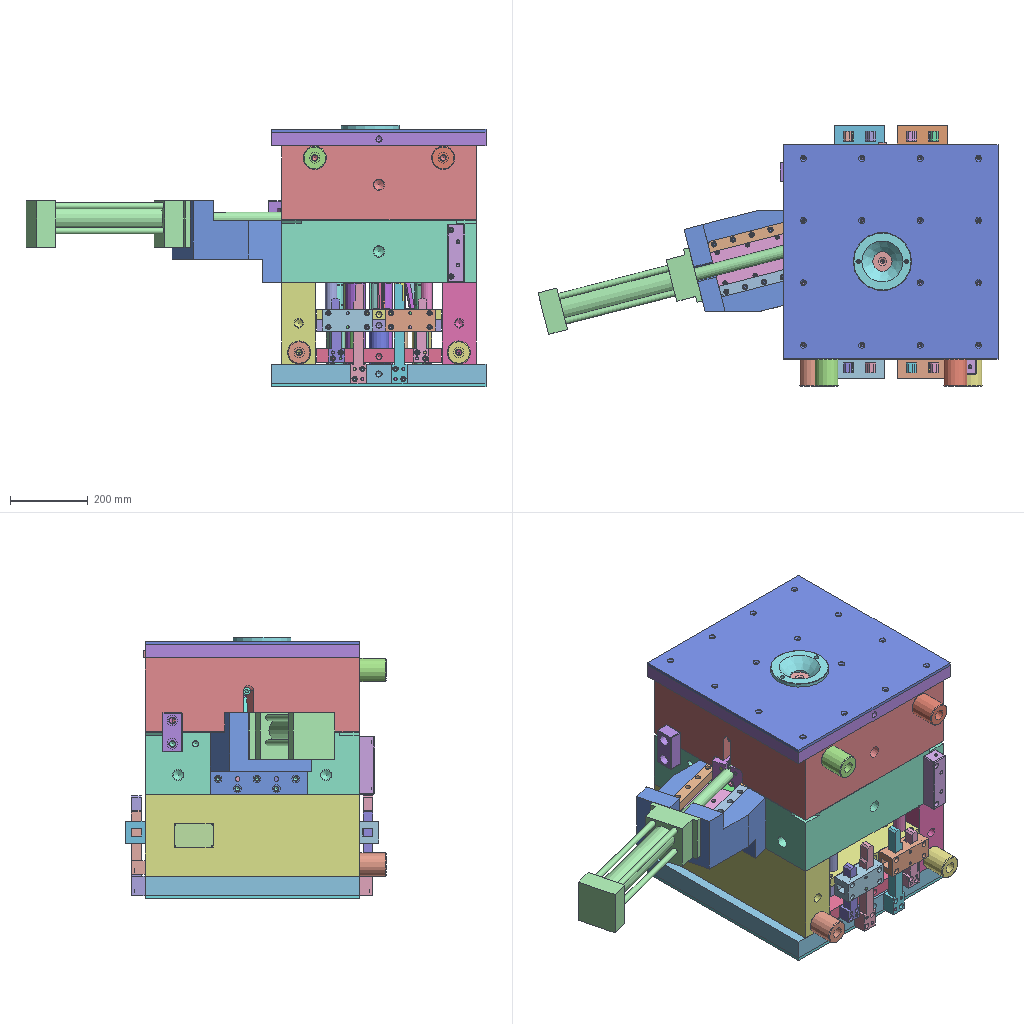Assembly | STEP file | 180 different items | 180 placed | box 1182 x 670 x 672 mm
Parts list (item | name | quantity | size | volume):
1 | stop_rings_id14_x_t | x1 | 20 x 20 x 5 mm | 1313 mm3
2 | stop_rings_id370_x_t | x1 | 20 x 20 x 5 mm | 1313 mm3
3 | stop_rings_id594_x_t | x1 | 20 x 20 x 5 mm | 1313 mm3
4 | stop_rings_id98_x_t | x1 | 20 x 20 x 5 mm | 1313 mm3
5 | 车灯-后视镜_id102_x_t | x1 | 9.556 x 9.556 x 88.278 mm | 4490 mm3
6 | 车灯-后视镜_id106_x_t | x1 | 320 x 550 x 25 mm | 3596280 mm3
7 | 车灯-后视镜_id10_x_t | x1 | 72 x 31.93 x 179.239 mm | 38387 mm3
8 | 车灯-后视镜_id110_x_t | x1 | 129 x 50 x 56 mm | 226318 mm3
9 | 车灯-后视镜_id114_x_t | x1 | 134.693 x 54.944 x 30.493 mm | 17624 mm3
10 | 车灯-后视镜_id118_x_t | x1 | 8 x 50 x 8 mm | 2507 mm3
11 | 车灯-后视镜_id122_x_t | x1 | 100 x 30 x 22 mm | 49982 mm3
12 | 车灯-后视镜_id126_x_t | x1 | 131.992 x 61.149 x 25 mm | 85679 mm3
13 | 车灯-后视镜_id130_x_t | x1 | 61 x 61 x 190 mm | 217774 mm3
14 | 车灯-后视镜_id134_x_t | x1 | 8 x 50 x 8 mm | 2507 mm3
15 | 车灯-后视镜_id138_x_t | x1 | 54.498 x 54.966 x 10 mm | 23790 mm3
16 | 车灯-后视镜_id142_x_t | x1 | 119.383 x 46.093 x 19.5 mm | 38380 mm3
17 | 车灯-后视镜_id146_x_t | x1 | 35 x 35 x 266 mm | 189704 mm3
18 | 车灯-后视镜_id150_x_t | x1 | 8 x 65 x 8 mm | 3261 mm3
19 | 车灯-后视镜_id154_x_t | x1 | 50 x 50 x 85 mm | 164490 mm3
20 | 车灯-后视镜_id158_x_t | x1 | 50.025 x 57.447 x 20 mm | 38834 mm3
21 | 车灯-后视镜_id162_x_t | x1 | 40 x 35 x 257 mm | 187577 mm3
22 | 车灯-后视镜_id166_x_t | x1 | 48 x 48 x 33 mm | 27966 mm3
23 | 车灯-后视镜_id170_x_t | x1 | 9.556 x 9.556 x 94.778 mm | 4817 mm3
24 | 车灯-后视镜_id174_x_t | x1 | 45 x 45 x 330 mm | 416787 mm3
25 | 车灯-后视镜_id178_x_t | x1 | 129 x 50 x 56 mm | 226318 mm3
26 | 车灯-后视镜_id182_x_t | x1 | 48.889 x 38.111 x 25.8 mm | 22170 mm3
27 | 车灯-后视镜_id186_x_t | x1 | 8 x 50 x 8 mm | 2507 mm3
28 | 车灯-后视镜_id18_x_t | x1 | 40 x 40 x 210 mm | 261823 mm3
29 | 车灯-后视镜_id190_x_t | x1 | 100 x 30 x 16.5 mm | 35524 mm3
30 | 车灯-后视镜_id194_x_t | x1 | 192.29 x 72.898 x 25 mm | 123539 mm3
31 | 车灯-后视镜_id198_x_t | x1 | 122.477 x 248.122 x 87.358 mm | 134816 mm3
32 | 车灯-后视镜_id202_x_t | x1 | 8 x 50 x 8 mm | 2507 mm3
33 | 车灯-后视镜_id206_x_t | x1 | 31.448 x 10.108 x 8 mm | 1557 mm3
34 | 车灯-后视镜_id210_x_t | x1 | 119.383 x 46.093 x 27 mm | 44427 mm3
35 | 车灯-后视镜_id214_x_t | x1 | 40 x 40 x 285 mm | 273765 mm3
36 | 车灯-后视镜_id218_x_t | x1 | 8 x 65 x 8 mm | 3261 mm3
37 | 车灯-后视镜_id222_x_t | x1 | 50 x 50 x 85 mm | 164490 mm3
38 | 车灯-后视镜_id226_x_t | x1 | 54.406 x 53.469 x 20 mm | 39812 mm3
39 | 车灯-后视镜_id22_x_t | x1 | 50 x 50 x 85 mm | 164490 mm3
40 | 车灯-后视镜_id230_x_t | x1 | 40 x 35 x 165 mm | 113527 mm3
41 | 车灯-后视镜_id234_x_t | x1 | 35 x 35 x 266 mm | 189704 mm3
42 | 车灯-后视镜_id238_x_t | x1 | 340.675 x 161.916 x 145 mm | 1865094 mm3
43 | 车灯-后视镜_id242_x_t | x1 | 54 x 54 x 53 mm | 49426 mm3
44 | 车灯-后视镜_id246_x_t | x1 | 129 x 50 x 56 mm | 226318 mm3
45 | 车灯-后视镜_id250_x_t | x1 | 180.044 x 59.602 x 42.214 mm | 28311 mm3
46 | 车灯-后视镜_id254_x_t | x1 | 8 x 65 x 8 mm | 3261 mm3
47 | 车灯-后视镜_id258_x_t | x1 | 25 x 50 x 18 mm | 16008 mm3
48 | 车灯-后视镜_id262_x_t | x1 | 226.748 x 84.296 x 25 mm | 147489 mm3
49 | 车灯-后视镜_id266_x_t | x1 | 8 x 50 x 8 mm | 2507 mm3
50 | 车灯-后视镜_id26_x_t | x1 | 84.183 x 23.326 x 319.699 mm | 124323 mm3
51 | 车灯-后视镜_id270_x_t | x1 | 36.435 x 10.457 x 8 mm | 1807 mm3
52 | 车灯-后视镜_id274_x_t | x1 | 33.319 x 37.519 x 48.057 mm | 14519 mm3
53 | 车灯-后视镜_id278_x_t | x1 | 48 x 48 x 33 mm | 27966 mm3
54 | 车灯-后视镜_id282_x_t | x1 | 8 x 65 x 8 mm | 3261 mm3
55 | 车灯-后视镜_id286_x_t | x1 | 50 x 50 x 210 mm | 409927 mm3
56 | 车灯-后视镜_id290_x_t | x1 | 64.479 x 55.577 x 20 mm | 48278 mm3
57 | 车灯-后视镜_id294_x_t | x1 | 122.477 x 248.122 x 87.358 mm | 134767 mm3
58 | 车灯-后视镜_id298_x_t | x1 | 149.9 x 149.9 x 33 mm | 429222 mm3
59 | 车灯-后视镜_id302_x_t | x1 | 40 x 35 x 165 mm | 113527 mm3
60 | 车灯-后视镜_id306_x_t | x1 | 40 x 40 x 285 mm | 273765 mm3
61 | 车灯-后视镜_id30_x_t | x1 | 54 x 54 x 53 mm | 49426 mm3
62 | 车灯-后视镜_id310_x_t | x1 | 80 x 12 x 12 mm | 9048 mm3
63 | 车灯-后视镜_id314_x_t | x1 | 45 x 45 x 330 mm | 416787 mm3
64 | 车灯-后视镜_id318_x_t | x1 | 40 x 35 x 165 mm | 113527 mm3
65 | 车灯-后视镜_id322_x_t | x1 | 81.604 x 38.677 x 31.456 mm | 5262 mm3
66 | 车灯-后视镜_id326_x_t | x1 | 8 x 50 x 8 mm | 2507 mm3
67 | 车灯-后视镜_id330_x_t | x1 | 30 x 100 x 16.5 mm | 35524 mm3
68 | 车灯-后视镜_id334_x_t | x1 | 178.639 x 104.251 x 61.239 mm | 236319 mm3
69 | 车灯-后视镜_id338_x_t | x1 | 8 x 50 x 8 mm | 2507 mm3
70 | 车灯-后视镜_id342_x_t | x1 | 10.152 x 35.922 x 8 mm | 1784 mm3
71 | 车灯-后视镜_id346_x_t | x1 | 8 x 8 x 16 mm | 739.323 mm3
72 | 车灯-后视镜_id34_x_t | x1 | 182.446 x 54.425 x 9.706 mm | 9470 mm3
73 | 车灯-后视镜_id350_x_t | x1 | 48 x 48 x 33 mm | 27966 mm3
74 | 车灯-后视镜_id354_x_t | x1 | 8 x 50 x 8 mm | 2507 mm3
75 | 车灯-后视镜_id358_x_t | x1 | 50 x 50 x 210 mm | 409927 mm3
76 | 车灯-后视镜_id362_x_t | x1 | 50.625 x 37.635 x 28 mm | 23645 mm3
77 | 车灯-后视镜_id366_x_t | x1 | - | 9620612 mm3
78 | 车灯-后视镜_id374_x_t | x1 | 44 x 40 x 150 mm | 242093 mm3
79 | 车灯-后视镜_id378_x_t | x1 | 35 x 25 x 20 mm | 16780 mm3
80 | 车灯-后视镜_id382_x_t | x1 | 40 x 40 x 285 mm | 273765 mm3
81 | 车灯-后视镜_id386_x_t | x1 | 80 x 12 x 12 mm | 9048 mm3
82 | 车灯-后视镜_id38_x_t | x1 | 320 x 550 x 30 mm | 4485754 mm3
83 | 车灯-后视镜_id390_x_t | x1 | 54 x 54 x 53 mm | 49426 mm3
84 | 车灯-后视镜_id394_x_t | x1 | 40 x 35 x 165 mm | 113527 mm3
85 | 车灯-后视镜_id398_x_t | x1 | 259.149 x 112.453 x 94.778 mm | 42702 mm3
86 | 车灯-后视镜_id402_x_t | x1 | 6.332 x 10 x 315.5 mm | 6416 mm3
87 | 车灯-后视镜_id406_x_t | x1 | 30 x 100 x 16.5 mm | 35524 mm3
88 | 车灯-后视镜_id410_x_t | x1 | 133.87 x 99.984 x 67.76 mm | 199506 mm3
89 | 车灯-后视镜_id414_x_t | x1 | 8 x 65 x 8 mm | 3261 mm3
90 | 车灯-后视镜_id418_x_t | x1 | 8.91 x 32.338 x 7 mm | 1230 mm3
91 | 车灯-后视镜_id422_x_t | x1 | 688.746 x 238.169 x 120 mm | 2911913 mm3
92 | 车灯-后视镜_id426_x_t | x1 | 45 x 45 x 330 mm | 416787 mm3
93 | 车灯-后视镜_id42_x_t | x1 | 129 x 50 x 56 mm | 226318 mm3
94 | 车灯-后视镜_id430_x_t | x1 | 8 x 50 x 8 mm | 2507 mm3
95 | 车灯-后视镜_id434_x_t | x1 | 50 x 50 x 210 mm | 409927 mm3
96 | 车灯-后视镜_id438_x_t | x1 | 44.639 x 37.217 x 28 mm | 22385 mm3
97 | 车灯-后视镜_id442_x_t | x1 | 197.778 x 377 x 123 mm | 135916 mm3
98 | 车灯-后视镜_id446_x_t | x1 | 35 x 35 x 266 mm | 189704 mm3
99 | 车灯-后视镜_id450_x_t | x1 | 60 x 70 x 60 mm | 173692 mm3
100 | 车灯-后视镜_id454_x_t | x1 | 35 x 25 x 20 mm | 16780 mm3
101 | 车灯-后视镜_id458_x_t | x1 | 45 x 45 x 330 mm | 416787 mm3
102 | 车灯-后视镜_id462_x_t | x1 | 53.642 x 50.81 x 378.343 mm | 173095 mm3
103 | 车灯-后视镜_id466_x_t | x1 | 550 x 550 x 50 mm | 14539056 mm3
104 | 车灯-后视镜_id46_x_t | x1 | 32.198 x 38.885 x 23 mm | 17479 mm3
105 | 车灯-后视镜_id470_x_t | x1 | 40 x 35 x 257 mm | 187577 mm3
106 | 车灯-后视镜_id474_x_t | x1 | 179.972 x 53.773 x 9.672 mm | 9329 mm3
107 | 车灯-后视镜_id478_x_t | x1 | 281.237 x 377 x 129.698 mm | 171076 mm3
108 | 车灯-后视镜_id482_x_t | x1 | 35 x 35 x 80 mm | 41432 mm3
109 | 车灯-后视镜_id486_x_t | x1 | 167.24 x 56.347 x 33.937 mm | 25779 mm3
110 | 车灯-后视镜_id490_x_t | x1 | 8 x 50 x 8 mm | 2507 mm3
111 | 车灯-后视镜_id494_x_t | x1 | 100 x 30 x 22 mm | 49982 mm3
112 | 车灯-后视镜_id498_x_t | x1 | 281.721 x 260 x 210 mm | 5973033 mm3
113 | 车灯-后视镜_id502_x_t | x1 | 500 x 550 x 190 mm | 33080670 mm3
114 | 车灯-后视镜_id506_x_t | x1 | 8 x 50 x 8 mm | 2507 mm3
115 | 车灯-后视镜_id50_x_t | x1 | 8 x 50 x 8 mm | 2507 mm3
116 | 车灯-后视镜_id510_x_t | x1 | 50 x 50 x 210 mm | 409927 mm3
117 | 车灯-后视镜_id514_x_t | x1 | 37.194 x 48.439 x 28 mm | 23466 mm3
118 | 车灯-后视镜_id518_x_t | x1 | 280 x 161 x 111 mm | 104739 mm3
119 | 车灯-后视镜_id522_x_t | x1 | 88 x 550 x 210 mm | 9957650 mm3
120 | 车灯-后视镜_id526_x_t | x1 | 60 x 70 x 60 mm | 173692 mm3
121 | 车灯-后视镜_id530_x_t | x1 | 35 x 25 x 20 mm | 16780 mm3
122 | 车灯-后视镜_id534_x_t | x1 | 21.278 x 54.656 x 325.478 mm | 91960 mm3
123 | 车灯-后视镜_id538_x_t | x1 | 40 x 40 x 285 mm | 273765 mm3
124 | 车灯-后视镜_id542_x_t | x1 | 40 x 35 x 257 mm | 187577 mm3
125 | 车灯-后视镜_id546_x_t | x1 | 125.408 x 39.857 x 9.556 mm | 6500 mm3
126 | 车灯-后视镜_id54_x_t | x1 | 100 x 30 x 16.5 mm | 35524 mm3
127 | 车灯-后视镜_id550_x_t | x1 | 280 x 377 x 150.384 mm | 11421529 mm3
128 | 车灯-后视镜_id554_x_t | x1 | 35 x 35 x 80 mm | 41432 mm3
129 | 车灯-后视镜_id558_x_t | x1 | 73.047 x 36.358 x 27.14 mm | 5259 mm3
130 | 车灯-后视镜_id562_x_t | x1 | 8 x 50 x 8 mm | 2507 mm3
131 | 车灯-后视镜_id566_x_t | x1 | 30 x 100 x 22 mm | 49982 mm3
132 | 车灯-后视镜_id570_x_t | x1 | 56.564 x 86.901 x 79.724 mm | 59028 mm3
133 | 车灯-后视镜_id574_x_t | x1 | 61 x 61 x 190 mm | 217774 mm3
134 | 车灯-后视镜_id578_x_t | x1 | 8 x 50 x 8 mm | 2507 mm3
135 | 车灯-后视镜_id582_x_t | x1 | 550 x 550 x 8 mm | 2264649 mm3
136 | 车灯-后视镜_id586_x_t | x1 | 37.285 x 49.936 x 28 mm | 23540 mm3
137 | 车灯-后视镜_id58_x_t | x1 | 125 x 59.346 x 25 mm | 80625 mm3
138 | 车灯-后视镜_id590_x_t | x1 | 6.638 x 10 x 131.059 mm | 3645 mm3
139 | 车灯-后视镜_id598_x_t | x1 | 60 x 70 x 60 mm | 173692 mm3
140 | 车灯-后视镜_id602_x_t | x1 | 35 x 25 x 20 mm | 16780 mm3
141 | 车灯-后视镜_id606_x_t | x1 | 15.208 x 52.995 x 313.531 mm | 58140 mm3
142 | 车灯-后视镜_id610_x_t | x1 | 48 x 48 x 33 mm | 27966 mm3
143 | 车灯-后视镜_id614_x_t | x1 | 40 x 35 x 257 mm | 187577 mm3
144 | 车灯-后视镜_id618_x_t | x1 | 125.408 x 39.857 x 9.556 mm | 6500 mm3
145 | 车灯-后视镜_id622_x_t | x1 | 500 x 550 x 160 mm | 32899557 mm3
146 | 车灯-后视镜_id626_x_t | x1 | 35 x 35 x 80 mm | 41432 mm3
147 | 车灯-后视镜_id62_x_t | x1 | 61 x 61 x 190 mm | 217774 mm3
148 | 车灯-后视镜_id630_x_t | x1 | 156.791 x 56.039 x 26.254 mm | 19026 mm3
149 | 车灯-后视镜_id634_x_t | x1 | 8 x 65 x 8 mm | 3261 mm3
150 | 车灯-后视镜_id638_x_t | x1 | 30 x 100 x 22 mm | 49982 mm3
151 | 车灯-后视镜_id642_x_t | x1 | 152.531 x 146.332 x 12 mm | 183119 mm3
152 | 车灯-后视镜_id646_x_t | x1 | 550 x 550 x 35 mm | 10040225 mm3
153 | 车灯-后视镜_id650_x_t | x1 | 8 x 50 x 8 mm | 2507 mm3
154 | 车灯-后视镜_id654_x_t | x1 | 550 x 550 x 8 mm | 2381998 mm3
155 | 车灯-后视镜_id658_x_t | x1 | 55.522 x 50.883 x 10 mm | 21930 mm3
156 | 车灯-后视镜_id662_x_t | x1 | 10 x 10 x 138.616 mm | 4062 mm3
157 | 车灯-后视镜_id666_x_t | x1 | 54 x 54 x 53 mm | 49426 mm3
158 | 车灯-后视镜_id66_x_t | x1 | 8 x 65 x 8 mm | 3261 mm3
159 | 车灯-后视镜_id670_x_t | x1 | 60 x 70 x 60 mm | 173692 mm3
160 | 车灯-后视镜_id674_x_t | x1 | 50 x 50 x 85 mm | 164490 mm3
161 | 车灯-后视镜_id678_x_t | x1 | 70.106 x 20.475 x 302.011 mm | 62813 mm3
162 | 车灯-后视镜_id682_x_t | x1 | 88 x 550 x 210 mm | 9957597 mm3
163 | 车灯-后视镜_id686_x_t | x1 | 24.107 x 64.242 x 19.839 mm | 3383 mm3
164 | 车灯-后视镜_id690_x_t | x1 | 320 x 550 x 35 mm | 4960596 mm3
165 | 车灯-后视镜_id694_x_t | x1 | 35 x 35 x 80 mm | 41432 mm3
166 | 车灯-后视镜_id698_x_t | x1 | 64.214 x 40.022 x 86 mm | 109388 mm3
167 | 车灯-后视镜_id6_x_t | x1 | 49.536 x 50.464 x 10 mm | 19050 mm3
168 | 车灯-后视镜_id702_x_t | x1 | 8 x 65 x 8 mm | 3261 mm3
169 | 车灯-后视镜_id706_x_t | x1 | 25 x 50 x 13 mm | 11607 mm3
170 | 车灯-后视镜_id70_x_t | x1 | 35 x 50 x 100 mm | 146008 mm3
171 | 车灯-后视镜_id710_x_t | x1 | 214.417 x 153.693 x 12 mm | 250941 mm3
172 | 车灯-后视镜_id714_x_t | x1 | 61 x 61 x 190 mm | 217774 mm3
173 | 车灯-后视镜_id718_x_t | x1 | 8 x 50 x 8 mm | 2507 mm3
174 | 车灯-后视镜_id722_x_t | x1 | 65 x 337.5 x 148.701 mm | 402158 mm3
175 | 车灯-后视镜_id74_x_t | x1 | 54.406 x 53.469 x 10 mm | 23010 mm3
176 | 车灯-后视镜_id78_x_t | x1 | 143.857 x 68.896 x 72 mm | 222992 mm3
177 | 车灯-后视镜_id82_x_t | x1 | 35 x 35 x 266 mm | 189704 mm3
178 | 车灯-后视镜_id86_x_t | x1 | 0.5 x 100 x 60 mm | 2994 mm3
179 | 车灯-后视镜_id90_x_t | x1 | 50 x 50 x 85 mm | 164490 mm3
180 | 车灯-后视镜_id94_x_t | x1 | 56.149 x 59.861 x 20 mm | 45570 mm3